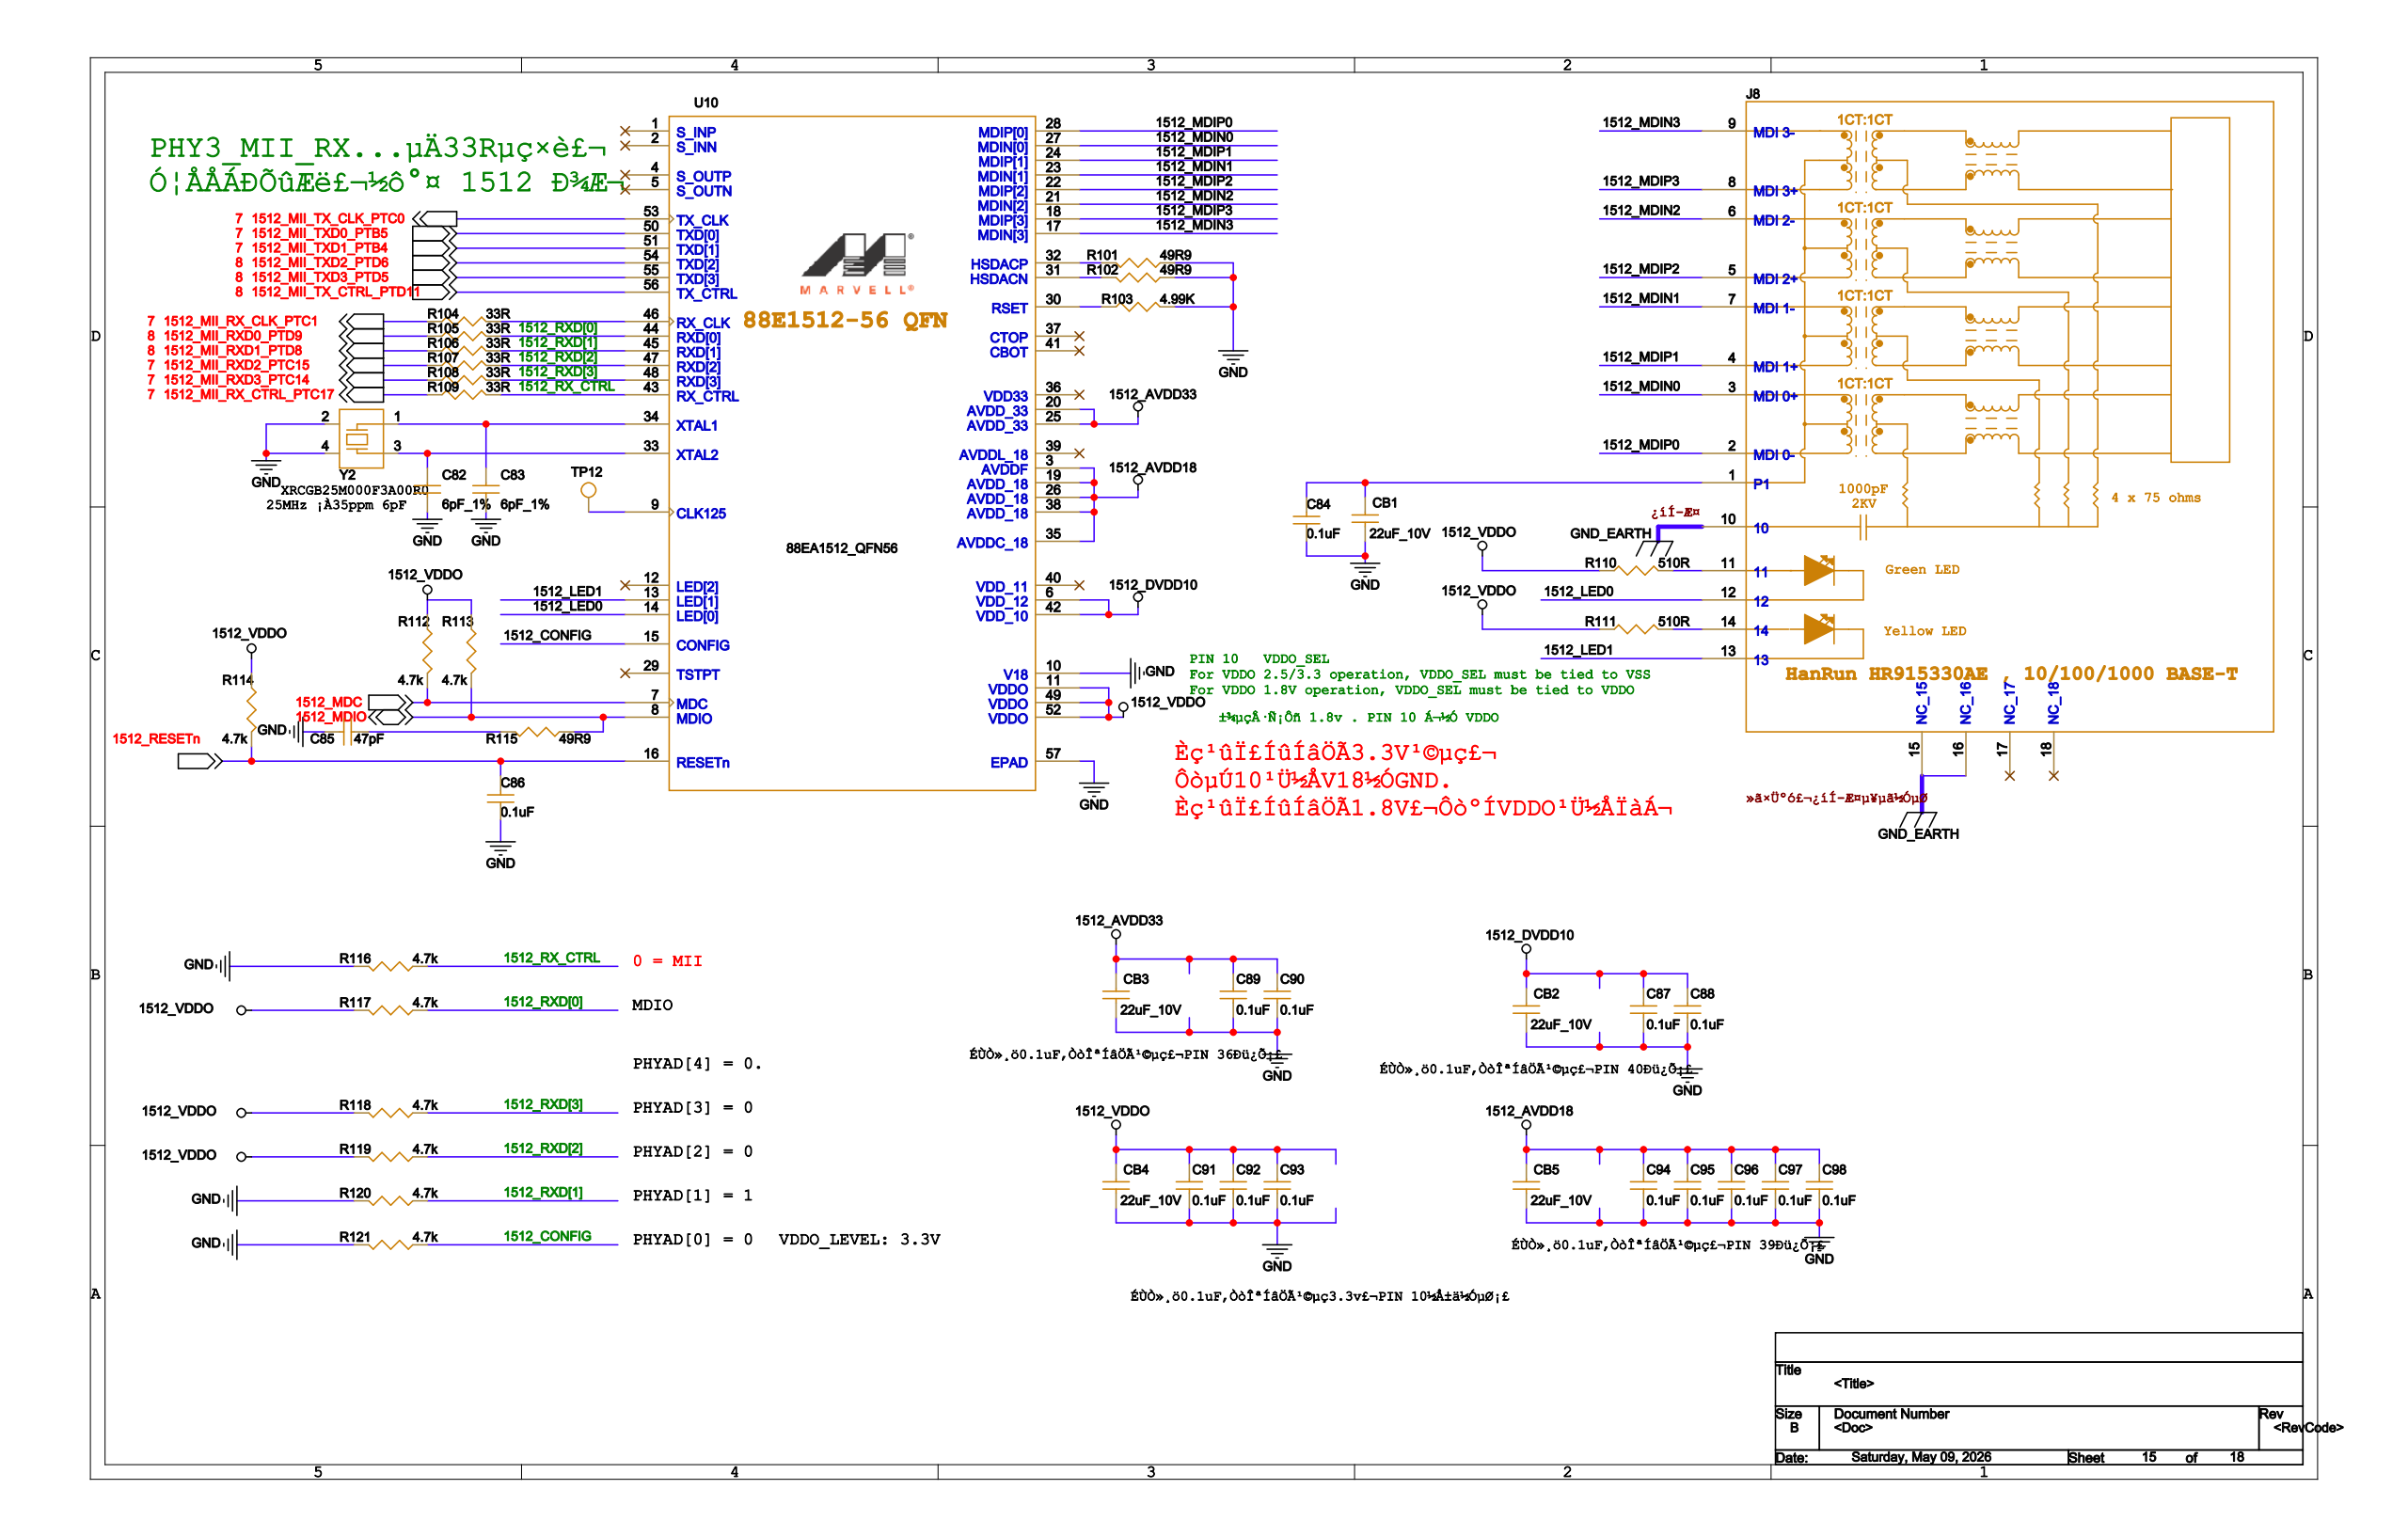Circuit board | Cadence Allegro | 330 parts | 215 nets | one sheet of the schematic
Parts on this sheet (reference | value | footprint):
C82 | 6pF_1% | 0402
C83 | 6pF_1% | 0402
C84 | 0.1uF | 0402
C85 | 47pF | 0402
C86 | 0.1uF | 0402
C87 | 0.1uF | 0402
C88 | 0.1uF | 0402
C89 | 0.1uF | 0402
C90 | 0.1uF | 0402
C91 | 0.1uF | 0402
C92 | 0.1uF | 0402
C93 | 0.1uF | 0402
C94 | 0.1uF | 0402
C95 | 0.1uF | 0402
C96 | 0.1uF | 0402
C97 | 0.1uF | 0402
C98 | 0.1uF | 0402
CB1 | 22uF_10V | 0805
CB2 | 22uF_10V | 1206
CB3 | 22uF_10V | 1206
CB4 | 22uF_10V | 1206
CB5 | 22uF_10V | 1206
J8 | HR915330AE | HR915330AE
R101 | 49R9 | 0402
R102 | 49R9 | 0402
R103 | 4.99K | 0402
R104 | 33R | 0402
R105 | 33R | 0402
R106 | 33R | 0402
R107 | 33R | 0402
R108 | 33R | 0402
R109 | 33R | 0402
R110 | 510R | 0402
R111 | 510R | 0402
R112 | 4.7K | 0402
R113 | 4.7K | 0402
R114 | 4.7K | 0402
R115 | 49R9 | 0402
R116 | 4.7K | 0402
R117 | 4.7K | 0402
R118 | 4.7K | 0402
R119 | 4.7K | 0402
R120 | 4.7K | 0402
R121 | 4.7K | 0402
TP12 | TP | S0400CI
U10 | 88EA1512_QFN56 | QFN50P800X800X100-56N_180X180EP
Y2 | XRCGB25M000F3A00R00 | CRYSTAL_SM
Nets of these parts (net: part-pin ...):
GND: C82-2 C83-2 C84-1 C85-2 C86-1 C87-2 C88-2 C89-2 C90-2 C91-2 C92-2 C93-2 C94-2 C95-2 C96-2 C97-2 C98-2 CB1-2 CB2-2 CB3-2 CB4-2 CB5-2 R101-2 R102-2 R103-2 R116-1 R120-1 R121-1 Y2-2 Y2-4 U10-10 U10-57
1512_DVDD10: C87-1 C88-1 CB2-1 U10-6 U10-42
1512_AVDD18: C94-1 C95-1 C96-1 C97-1 C98-1 CB5-1 U10-3 U10-19 U10-26 U10-35 U10-38
1512_AVDD33: C89-1 C90-1 CB3-1 U10-20 U10-25
1512_VDDO: C91-1 C92-1 C93-1 CB4-1 R110-1 R111-1 R112-2 R113-2 R114-2 R117-1 R118-1 R119-1 U10-11 U10-49 U10-52
GND_EARTH: J8-10 J8-15 J8-16
1512_MDC: R112-1 U10-7
1512_MDIO: R113-1 R115-2 U10-8
1512_RESETN: C86-2 R114-1 U10-16
1512_RX_CTRL: R109-2 R116-2 U10-43
1512_RXD[0]: R105-2 R117-2 U10-44
1512_RXD[3]: R108-2 R118-2 U10-48
1512_RXD[2]: R107-2 R119-2 U10-47
1512_RXD[1]: R106-2 R120-2 U10-45
1512_CONFIG: R121-2 U10-15
N1754463: R101-1 U10-32
N1754505: R102-1 U10-31
N1755361: C85-1 R115-1
N1754569: R103-1 U10-30
1512_MII_RX_CLK_PTC1: R104-1
N1754617: R104-2 U10-46
1512_MII_RXD0_PTD9: R105-1
1512_MII_RXD1_PTD8: R106-1
1512_MII_RXD2_PTC15: R107-1
1512_MII_RXD3_PTC14: R108-1
1512_MII_RX_CTRL_PTC17: R109-1
1512_MII_TXD1_PTB4: U10-51
1512_MII_TXD0_PTB5: U10-50
1512_MII_TX_CLK_PTC0: U10-53
1512_MII_TXD3_PTD5: U10-55
1512_MII_TXD2_PTD6: U10-54
1512_MII_TX_CTRL_PTD11: U10-56
N1755135: J8-11 R110-2
N1755225: J8-14 R111-2
N1755027: TP12-1 U10-9
1512_LED0: J8-12 U10-14
1512_LED1: J8-13 U10-13
1512_MDIN0: J8-3 U10-27
1512_MDIN1: J8-7 U10-23
1512_MDIN2: J8-6 U10-21
1512_MDIN3: J8-9 U10-17
1512_MDIP0: J8-2 U10-28
1512_MDIP1: J8-4 U10-24
1512_MDIP2: J8-5 U10-22
1512_MDIP3: J8-8 U10-18
N1754871: C83-1 Y2-1 U10-34
N1754891: C82-1 Y2-3 U10-33
N1754991: C84-2 CB1-1 J8-1